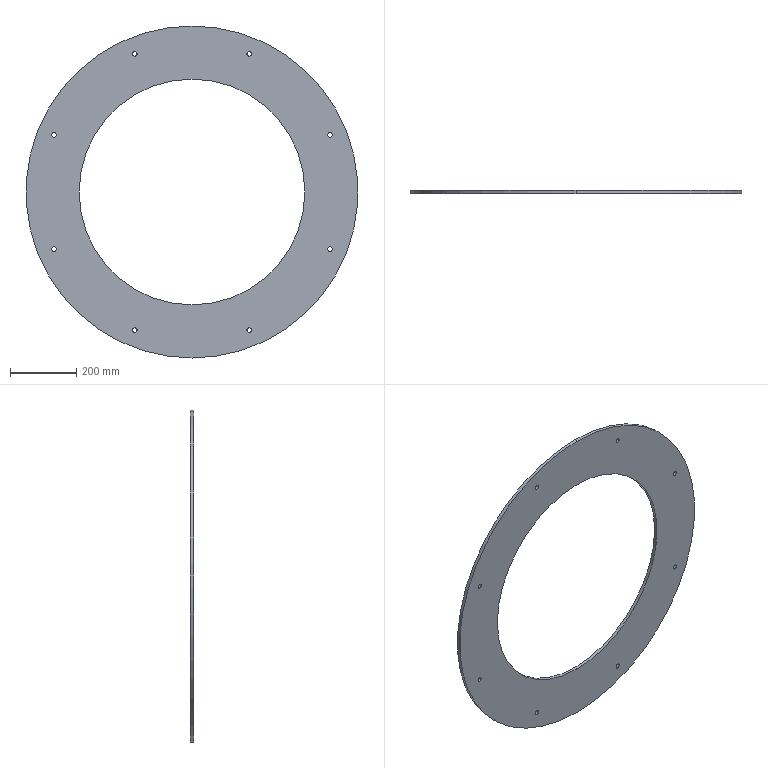Part | SolidWorks | features Extrusion 1, HoleWzd 1 | 1 solid | 22 faces | box 1000 x 10 x 1000 mm | volume 4210849 mm3 | cylinder 20 | plane 2 | commonest cylinder face diameters 13.5 x16 680 x2 1000 x2
STEP:
#1=CARTESIAN_POINT('',(172.208,-5.,-422.496));
#2=VERTEX_POINT('',#1);
#3=CARTESIAN_POINT('',(172.208,-5.,-408.996));
#4=VERTEX_POINT('',#3);
#5=CARTESIAN_POINT('',(172.208,-5.,-415.746));
#6=DIRECTION('',(0.,1.,0.));
#7=DIRECTION('',(0.,0.,1.));
#8=AXIS2_PLACEMENT_3D('',#5,#6,#7);
#9=CIRCLE('',#8,6.75);
#10=EDGE_CURVE('',#2,#4,#9,.T.);
#11=ORIENTED_EDGE('',*,*,#10,.F.);
#12=CARTESIAN_POINT('',(172.208,5.,-422.496));
#13=VERTEX_POINT('',#12);
#14=CARTESIAN_POINT('',(172.208,5.,-422.496));
#15=DIRECTION('',(0.,1.,0.));
#16=VECTOR('',#15,1000.);
#17=LINE('',#14,#16);
#18=EDGE_CURVE('',#2,#13,#17,.T.);
#19=ORIENTED_EDGE('',*,*,#18,.T.);
#20=CARTESIAN_POINT('',(172.208,5.,-408.996));
#21=VERTEX_POINT('',#20);
#22=CARTESIAN_POINT('',(172.208,5.,-415.746));
#23=DIRECTION('',(0.,1.,0.));
#24=DIRECTION('',(0.,0.,1.));
#25=AXIS2_PLACEMENT_3D('',#22,#23,#24);
#26=CIRCLE('',#25,6.75);
#27=EDGE_CURVE('',#13,#21,#26,.T.);
#28=ORIENTED_EDGE('',*,*,#27,.T.);
#29=CARTESIAN_POINT('',(172.208,5.,-408.996));
#30=DIRECTION('',(0.,1.,0.));
#31=VECTOR('',#30,1000.);
#32=LINE('',#29,#31);
#33=EDGE_CURVE('',#4,#21,#32,.T.);
#34=ORIENTED_EDGE('',*,*,#33,.F.);
#35=EDGE_LOOP('',(#11,#19,#28,#34));
#36=FACE_OUTER_BOUND('',#35,.T.);
#37=CARTESIAN_POINT('',(172.208,5.,-415.746));
#38=DIRECTION('',(0.,1.,0.));
#39=DIRECTION('',(0.,0.,1.));
#40=AXIS2_PLACEMENT_3D('',#37,#38,#39);
#41=CYLINDRICAL_SURFACE('',#40,6.75);
#42=ADVANCED_FACE('',(#36),#41,.F.);
#43=CARTESIAN_POINT('',(415.746,-5.,-178.958));
#44=VERTEX_POINT('',#43);
#45=CARTESIAN_POINT('',(415.746,-5.,-165.458));
#46=VERTEX_POINT('',#45);
#47=CARTESIAN_POINT('',(415.746,-5.,-172.208));
#48=DIRECTION('',(0.,1.,0.));
#49=DIRECTION('',(0.,0.,1.));
#50=AXIS2_PLACEMENT_3D('',#47,#48,#49);
#51=CIRCLE('',#50,6.75);
#52=EDGE_CURVE('',#44,#46,#51,.T.);
#53=ORIENTED_EDGE('',*,*,#52,.F.);
#54=CARTESIAN_POINT('',(415.746,5.,-178.958));
#55=VERTEX_POINT('',#54);
#56=CARTESIAN_POINT('',(415.746,5.,-178.958));
#57=DIRECTION('',(0.,1.,0.));
#58=VECTOR('',#57,1000.);
#59=LINE('',#56,#58);
#60=EDGE_CURVE('',#44,#55,#59,.T.);
#61=ORIENTED_EDGE('',*,*,#60,.T.);
#62=CARTESIAN_POINT('',(415.746,5.,-165.458));
#63=VERTEX_POINT('',#62);
#64=CARTESIAN_POINT('',(415.746,5.,-172.208));
#65=DIRECTION('',(0.,1.,0.));
#66=DIRECTION('',(0.,0.,1.));
#67=AXIS2_PLACEMENT_3D('',#64,#65,#66);
#68=CIRCLE('',#67,6.75);
#69=EDGE_CURVE('',#55,#63,#68,.T.);
#70=ORIENTED_EDGE('',*,*,#69,.T.);
#71=CARTESIAN_POINT('',(415.746,5.,-165.458));
#72=DIRECTION('',(0.,1.,0.));
#73=VECTOR('',#72,1000.);
#74=LINE('',#71,#73);
#75=EDGE_CURVE('',#46,#63,#74,.T.);
#76=ORIENTED_EDGE('',*,*,#75,.F.);
#77=EDGE_LOOP('',(#53,#61,#70,#76));
#78=FACE_OUTER_BOUND('',#77,.T.);
#79=CARTESIAN_POINT('',(415.746,5.,-172.208));
#80=DIRECTION('',(0.,1.,0.));
#81=DIRECTION('',(0.,0.,1.));
#82=AXIS2_PLACEMENT_3D('',#79,#80,#81);
#83=CYLINDRICAL_SURFACE('',#82,6.75);
#84=ADVANCED_FACE('',(#78),#83,.F.);
#85=CARTESIAN_POINT('',(415.746,-5.,165.458));
#86=VERTEX_POINT('',#85);
#87=CARTESIAN_POINT('',(415.746,-5.,178.958));
#88=VERTEX_POINT('',#87);
#89=CARTESIAN_POINT('',(415.746,-5.,172.208));
#90=DIRECTION('',(0.,1.,0.));
#91=DIRECTION('',(0.,0.,1.));
#92=AXIS2_PLACEMENT_3D('',#89,#90,#91);
#93=CIRCLE('',#92,6.75);
#94=EDGE_CURVE('',#86,#88,#93,.T.);
#95=ORIENTED_EDGE('',*,*,#94,.F.);
#96=CARTESIAN_POINT('',(415.746,5.,165.458));
#97=VERTEX_POINT('',#96);
#98=CARTESIAN_POINT('',(415.746,5.,165.458));
#99=DIRECTION('',(0.,1.,0.));
#100=VECTOR('',#99,1000.);
#101=LINE('',#98,#100);
#102=EDGE_CURVE('',#86,#97,#101,.T.);
#103=ORIENTED_EDGE('',*,*,#102,.T.);
#104=CARTESIAN_POINT('',(415.746,5.,178.958));
#105=VERTEX_POINT('',#104);
#106=CARTESIAN_POINT('',(415.746,5.,172.208));
#107=DIRECTION('',(0.,1.,0.));
#108=DIRECTION('',(0.,0.,1.));
#109=AXIS2_PLACEMENT_3D('',#106,#107,#108);
#110=CIRCLE('',#109,6.75);
#111=EDGE_CURVE('',#97,#105,#110,.T.);
#112=ORIENTED_EDGE('',*,*,#111,.T.);
#113=CARTESIAN_POINT('',(415.746,5.,178.958));
#114=DIRECTION('',(0.,1.,0.));
#115=VECTOR('',#114,1000.);
#116=LINE('',#113,#115);
#117=EDGE_CURVE('',#88,#105,#116,.T.);
#118=ORIENTED_EDGE('',*,*,#117,.F.);
#119=EDGE_LOOP('',(#95,#103,#112,#118));
#120=FACE_OUTER_BOUND('',#119,.T.);
#121=CARTESIAN_POINT('',(415.746,5.,172.208));
#122=DIRECTION('',(0.,1.,0.));
#123=DIRECTION('',(0.,0.,1.));
#124=AXIS2_PLACEMENT_3D('',#121,#122,#123);
#125=CYLINDRICAL_SURFACE('',#124,6.75);
#126=ADVANCED_FACE('',(#120),#125,.F.);
#127=CARTESIAN_POINT('',(172.208,-5.,408.996));
#128=VERTEX_POINT('',#127);
#129=CARTESIAN_POINT('',(172.208,-5.,422.496));
#130=VERTEX_POINT('',#129);
#131=CARTESIAN_POINT('',(172.208,-5.,415.746));
#132=DIRECTION('',(0.,1.,0.));
#133=DIRECTION('',(0.,0.,1.));
#134=AXIS2_PLACEMENT_3D('',#131,#132,#133);
#135=CIRCLE('',#134,6.75);
#136=EDGE_CURVE('',#128,#130,#135,.T.);
#137=ORIENTED_EDGE('',*,*,#136,.F.);
#138=CARTESIAN_POINT('',(172.208,5.,408.996));
#139=VERTEX_POINT('',#138);
#140=CARTESIAN_POINT('',(172.208,5.,408.996));
#141=DIRECTION('',(0.,1.,0.));
#142=VECTOR('',#141,1000.);
#143=LINE('',#140,#142);
#144=EDGE_CURVE('',#128,#139,#143,.T.);
#145=ORIENTED_EDGE('',*,*,#144,.T.);
#146=CARTESIAN_POINT('',(172.208,5.,422.496));
#147=VERTEX_POINT('',#146);
#148=CARTESIAN_POINT('',(172.208,5.,415.746));
#149=DIRECTION('',(0.,1.,0.));
#150=DIRECTION('',(0.,0.,1.));
#151=AXIS2_PLACEMENT_3D('',#148,#149,#150);
#152=CIRCLE('',#151,6.75);
#153=EDGE_CURVE('',#139,#147,#152,.T.);
#154=ORIENTED_EDGE('',*,*,#153,.T.);
#155=CARTESIAN_POINT('',(172.208,5.,422.496));
#156=DIRECTION('',(0.,1.,0.));
#157=VECTOR('',#156,1000.);
#158=LINE('',#155,#157);
#159=EDGE_CURVE('',#130,#147,#158,.T.);
#160=ORIENTED_EDGE('',*,*,#159,.F.);
#161=EDGE_LOOP('',(#137,#145,#154,#160));
#162=FACE_OUTER_BOUND('',#161,.T.);
#163=CARTESIAN_POINT('',(172.208,5.,415.746));
#164=DIRECTION('',(0.,1.,0.));
#165=DIRECTION('',(0.,0.,1.));
#166=AXIS2_PLACEMENT_3D('',#163,#164,#165);
#167=CYLINDRICAL_SURFACE('',#166,6.75);
#168=ADVANCED_FACE('',(#162),#167,.F.);
#169=CARTESIAN_POINT('',(-172.208,-5.,408.996));
#170=VERTEX_POINT('',#169);
#171=CARTESIAN_POINT('',(-172.208,-5.,422.496));
#172=VERTEX_POINT('',#171);
#173=CARTESIAN_POINT('',(-172.208,-5.,415.746));
#174=DIRECTION('',(0.,1.,0.));
#175=DIRECTION('',(0.,0.,1.));
#176=AXIS2_PLACEMENT_3D('',#173,#174,#175);
#177=CIRCLE('',#176,6.75);
#178=EDGE_CURVE('',#170,#172,#177,.T.);
#179=ORIENTED_EDGE('',*,*,#178,.F.);
#180=CARTESIAN_POINT('',(-172.208,5.,408.996));
#181=VERTEX_POINT('',#180);
#182=CARTESIAN_POINT('',(-172.208,5.,408.996));
#183=DIRECTION('',(0.,1.,0.));
#184=VECTOR('',#183,1000.);
#185=LINE('',#182,#184);
#186=EDGE_CURVE('',#170,#181,#185,.T.);
#187=ORIENTED_EDGE('',*,*,#186,.T.);
#188=CARTESIAN_POINT('',(-172.208,5.,422.496));
#189=VERTEX_POINT('',#188);
#190=CARTESIAN_POINT('',(-172.208,5.,415.746));
#191=DIRECTION('',(0.,1.,0.));
#192=DIRECTION('',(0.,0.,1.));
#193=AXIS2_PLACEMENT_3D('',#190,#191,#192);
#194=CIRCLE('',#193,6.75);
#195=EDGE_CURVE('',#181,#189,#194,.T.);
#196=ORIENTED_EDGE('',*,*,#195,.T.);
#197=CARTESIAN_POINT('',(-172.208,5.,422.496));
#198=DIRECTION('',(0.,1.,0.));
#199=VECTOR('',#198,1000.);
#200=LINE('',#197,#199);
#201=EDGE_CURVE('',#172,#189,#200,.T.);
#202=ORIENTED_EDGE('',*,*,#201,.F.);
#203=EDGE_LOOP('',(#179,#187,#196,#202));
#204=FACE_OUTER_BOUND('',#203,.T.);
#205=CARTESIAN_POINT('',(-172.208,5.,415.746));
#206=DIRECTION('',(0.,1.,0.));
#207=DIRECTION('',(0.,0.,1.));
#208=AXIS2_PLACEMENT_3D('',#205,#206,#207);
#209=CYLINDRICAL_SURFACE('',#208,6.75);
#210=ADVANCED_FACE('',(#204),#209,.F.);
#211=CARTESIAN_POINT('',(-415.746,-5.,165.458));
#212=VERTEX_POINT('',#211);
#213=CARTESIAN_POINT('',(-415.746,-5.,178.958));
#214=VERTEX_POINT('',#213);
#215=CARTESIAN_POINT('',(-415.746,-5.,172.208));
#216=DIRECTION('',(0.,1.,0.));
#217=DIRECTION('',(0.,0.,1.));
#218=AXIS2_PLACEMENT_3D('',#215,#216,#217);
#219=CIRCLE('',#218,6.75);
#220=EDGE_CURVE('',#212,#214,#219,.T.);
#221=ORIENTED_EDGE('',*,*,#220,.F.);
#222=CARTESIAN_POINT('',(-415.746,5.,165.458));
#223=VERTEX_POINT('',#222);
#224=CARTESIAN_POINT('',(-415.746,5.,165.458));
#225=DIRECTION('',(0.,1.,0.));
#226=VECTOR('',#225,1000.);
#227=LINE('',#224,#226);
#228=EDGE_CURVE('',#212,#223,#227,.T.);
#229=ORIENTED_EDGE('',*,*,#228,.T.);
#230=CARTESIAN_POINT('',(-415.746,5.,178.958));
#231=VERTEX_POINT('',#230);
#232=CARTESIAN_POINT('',(-415.746,5.,172.208));
#233=DIRECTION('',(0.,1.,0.));
#234=DIRECTION('',(0.,0.,1.));
#235=AXIS2_PLACEMENT_3D('',#232,#233,#234);
#236=CIRCLE('',#235,6.75);
#237=EDGE_CURVE('',#223,#231,#236,.T.);
#238=ORIENTED_EDGE('',*,*,#237,.T.);
#239=CARTESIAN_POINT('',(-415.746,5.,178.958));
#240=DIRECTION('',(0.,1.,0.));
#241=VECTOR('',#240,1000.);
#242=LINE('',#239,#241);
#243=EDGE_CURVE('',#214,#231,#242,.T.);
#244=ORIENTED_EDGE('',*,*,#243,.F.);
#245=EDGE_LOOP('',(#221,#229,#238,#244));
#246=FACE_OUTER_BOUND('',#245,.T.);
#247=CARTESIAN_POINT('',(-415.746,5.,172.208));
#248=DIRECTION('',(0.,1.,0.));
#249=DIRECTION('',(0.,0.,1.));
#250=AXIS2_PLACEMENT_3D('',#247,#248,#249);
#251=CYLINDRICAL_SURFACE('',#250,6.75);
#252=ADVANCED_FACE('',(#246),#251,.F.);
#253=CARTESIAN_POINT('',(-415.746,-5.,-178.958));
#254=VERTEX_POINT('',#253);
#255=CARTESIAN_POINT('',(-415.746,-5.,-165.458));
#256=VERTEX_POINT('',#255);
#257=CARTESIAN_POINT('',(-415.746,-5.,-172.208));
#258=DIRECTION('',(0.,1.,0.));
#259=DIRECTION('',(0.,0.,1.));
#260=AXIS2_PLACEMENT_3D('',#257,#258,#259);
#261=CIRCLE('',#260,6.75);
#262=EDGE_CURVE('',#254,#256,#261,.T.);
#263=ORIENTED_EDGE('',*,*,#262,.F.);
#264=CARTESIAN_POINT('',(-415.746,5.,-178.958));
#265=VERTEX_POINT('',#264);
#266=CARTESIAN_POINT('',(-415.746,5.,-178.958));
#267=DIRECTION('',(0.,1.,0.));
#268=VECTOR('',#267,1000.);
#269=LINE('',#266,#268);
#270=EDGE_CURVE('',#254,#265,#269,.T.);
#271=ORIENTED_EDGE('',*,*,#270,.T.);
#272=CARTESIAN_POINT('',(-415.746,5.,-165.458));
#273=VERTEX_POINT('',#272);
#274=CARTESIAN_POINT('',(-415.746,5.,-172.208));
#275=DIRECTION('',(0.,1.,0.));
#276=DIRECTION('',(0.,0.,1.));
#277=AXIS2_PLACEMENT_3D('',#274,#275,#276);
#278=CIRCLE('',#277,6.75);
#279=EDGE_CURVE('',#265,#273,#278,.T.);
#280=ORIENTED_EDGE('',*,*,#279,.T.);
#281=CARTESIAN_POINT('',(-415.746,5.,-165.458));
#282=DIRECTION('',(0.,1.,0.));
#283=VECTOR('',#282,1000.);
#284=LINE('',#281,#283);
#285=EDGE_CURVE('',#256,#273,#284,.T.);
#286=ORIENTED_EDGE('',*,*,#285,.F.);
#287=EDGE_LOOP('',(#263,#271,#280,#286));
#288=FACE_OUTER_BOUND('',#287,.T.);
#289=CARTESIAN_POINT('',(-415.746,5.,-172.208));
#290=DIRECTION('',(0.,1.,0.));
#291=DIRECTION('',(0.,0.,1.));
#292=AXIS2_PLACEMENT_3D('',#289,#290,#291);
#293=CYLINDRICAL_SURFACE('',#292,6.75);
#294=ADVANCED_FACE('',(#288),#293,.F.);
#295=CARTESIAN_POINT('',(-172.208,-5.,-422.496));
#296=VERTEX_POINT('',#295);
#297=CARTESIAN_POINT('',(-172.208,-5.,-408.996));
#298=VERTEX_POINT('',#297);
#299=CARTESIAN_POINT('',(-172.208,-5.,-415.746));
#300=DIRECTION('',(0.,1.,0.));
#301=DIRECTION('',(0.,0.,1.));
#302=AXIS2_PLACEMENT_3D('',#299,#300,#301);
#303=CIRCLE('',#302,6.75);
#304=EDGE_CURVE('',#296,#298,#303,.T.);
#305=ORIENTED_EDGE('',*,*,#304,.F.);
#306=CARTESIAN_POINT('',(-172.208,5.,-422.496));
#307=VERTEX_POINT('',#306);
#308=CARTESIAN_POINT('',(-172.208,5.,-422.496));
#309=DIRECTION('',(0.,1.,0.));
#310=VECTOR('',#309,1000.);
#311=LINE('',#308,#310);
#312=EDGE_CURVE('',#296,#307,#311,.T.);
#313=ORIENTED_EDGE('',*,*,#312,.T.);
#314=CARTESIAN_POINT('',(-172.208,5.,-408.996));
#315=VERTEX_POINT('',#314);
#316=CARTESIAN_POINT('',(-172.208,5.,-415.746));
#317=DIRECTION('',(0.,1.,0.));
#318=DIRECTION('',(0.,0.,1.));
#319=AXIS2_PLACEMENT_3D('',#316,#317,#318);
#320=CIRCLE('',#319,6.75);
#321=EDGE_CURVE('',#307,#315,#320,.T.);
#322=ORIENTED_EDGE('',*,*,#321,.T.);
#323=CARTESIAN_POINT('',(-172.208,5.,-408.996));
#324=DIRECTION('',(0.,1.,0.));
#325=VECTOR('',#324,1000.);
#326=LINE('',#323,#325);
#327=EDGE_CURVE('',#298,#315,#326,.T.);
#328=ORIENTED_EDGE('',*,*,#327,.F.);
#329=EDGE_LOOP('',(#305,#313,#322,#328));
#330=FACE_OUTER_BOUND('',#329,.T.);
#331=CARTESIAN_POINT('',(-172.208,5.,-415.746));
#332=DIRECTION('',(0.,1.,0.));
#333=DIRECTION('',(0.,0.,1.));
#334=AXIS2_PLACEMENT_3D('',#331,#332,#333);
#335=CYLINDRICAL_SURFACE('',#334,6.75);
#336=ADVANCED_FACE('',(#330),#335,.F.);
#337=CARTESIAN_POINT('',(0.,5.,-340.));
#338=VERTEX_POINT('',#337);
#339=CARTESIAN_POINT('',(0.,5.,340.));
#340=VERTEX_POINT('',#339);
#341=CARTESIAN_POINT('',(0.,5.,0.));
#342=DIRECTION('',(0.,1.,0.));
#343=DIRECTION('',(0.,0.,1.));
#344=AXIS2_PLACEMENT_3D('',#341,#342,#343);
#345=CIRCLE('',#344,340.);
#346=EDGE_CURVE('',#338,#340,#345,.T.);
#347=ORIENTED_EDGE('',*,*,#346,.T.);
#348=CARTESIAN_POINT('',(0.,-5.,340.));
#349=VERTEX_POINT('',#348);
#350=CARTESIAN_POINT('',(0.,5.,340.));
#351=DIRECTION('',(0.,-1.,0.));
#352=VECTOR('',#351,1000.);
#353=LINE('',#350,#352);
#354=EDGE_CURVE('',#340,#349,#353,.T.);
#355=ORIENTED_EDGE('',*,*,#354,.T.);
#356=CARTESIAN_POINT('',(0.,-5.,-340.));
#357=VERTEX_POINT('',#356);
#358=CARTESIAN_POINT('',(0.,-5.,0.));
#359=DIRECTION('',(0.,1.,0.));
#360=DIRECTION('',(0.,0.,1.));
#361=AXIS2_PLACEMENT_3D('',#358,#359,#360);
#362=CIRCLE('',#361,340.);
#363=EDGE_CURVE('',#357,#349,#362,.T.);
#364=ORIENTED_EDGE('',*,*,#363,.F.);
#365=CARTESIAN_POINT('',(0.,5.,-340.));
#366=DIRECTION('',(0.,-1.,0.));
#367=VECTOR('',#366,1000.);
#368=LINE('',#365,#367);
#369=EDGE_CURVE('',#338,#357,#368,.T.);
#370=ORIENTED_EDGE('',*,*,#369,.F.);
#371=EDGE_LOOP('',(#347,#355,#364,#370));
#372=FACE_OUTER_BOUND('',#371,.T.);
#373=CARTESIAN_POINT('',(0.,5.,0.));
#374=DIRECTION('',(0.,-1.,0.));
#375=DIRECTION('',(0.,0.,-1.));
#376=AXIS2_PLACEMENT_3D('',#373,#374,#375);
#377=CYLINDRICAL_SURFACE('',#376,340.);
#378=ADVANCED_FACE('',(#372),#377,.F.);
#379=CARTESIAN_POINT('',(0.,5.,500.));
#380=VERTEX_POINT('',#379);
#381=CARTESIAN_POINT('',(0.,5.,-500.));
#382=VERTEX_POINT('',#381);
#383=CARTESIAN_POINT('',(0.,5.,0.));
#384=DIRECTION('',(0.,1.,0.));
#385=DIRECTION('',(0.,0.,1.));
#386=AXIS2_PLACEMENT_3D('',#383,#384,#385);
#387=CIRCLE('',#386,500.);
#388=EDGE_CURVE('',#380,#382,#387,.T.);
#389=ORIENTED_EDGE('',*,*,#388,.F.);
#390=CARTESIAN_POINT('',(0.,-5.,500.));
#391=VERTEX_POINT('',#390);
#392=CARTESIAN_POINT('',(0.,5.,500.));
#393=DIRECTION('',(0.,-1.,0.));
#394=VECTOR('',#393,1000.);
#395=LINE('',#392,#394);
#396=EDGE_CURVE('',#380,#391,#395,.T.);
#397=ORIENTED_EDGE('',*,*,#396,.T.);
#398=CARTESIAN_POINT('',(0.,-5.,-500.));
#399=VERTEX_POINT('',#398);
#400=CARTESIAN_POINT('',(0.,-5.,0.));
#401=DIRECTION('',(0.,1.,0.));
#402=DIRECTION('',(0.,0.,1.));
#403=AXIS2_PLACEMENT_3D('',#400,#401,#402);
#404=CIRCLE('',#403,500.);
#405=EDGE_CURVE('',#391,#399,#404,.T.);
#406=ORIENTED_EDGE('',*,*,#405,.T.);
#407=CARTESIAN_POINT('',(0.,5.,-500.));
#408=DIRECTION('',(0.,-1.,0.));
#409=VECTOR('',#408,1000.);
#410=LINE('',#407,#409);
#411=EDGE_CURVE('',#382,#399,#410,.T.);
#412=ORIENTED_EDGE('',*,*,#411,.F.);
#413=EDGE_LOOP('',(#389,#397,#406,#412));
#414=FACE_OUTER_BOUND('',#413,.T.);
#415=CARTESIAN_POINT('',(0.,5.,0.));
#416=DIRECTION('',(0.,-1.,0.));
#417=DIRECTION('',(0.,0.,-1.));
#418=AXIS2_PLACEMENT_3D('',#415,#416,#417);
#419=CYLINDRICAL_SURFACE('',#418,500.);
#420=ADVANCED_FACE('',(#414),#419,.T.);
#421=CARTESIAN_POINT('',(172.208,5.,-415.746));
#422=DIRECTION('',(0.,1.,0.));
#423=DIRECTION('',(0.,0.,1.));
#424=AXIS2_PLACEMENT_3D('',#421,#422,#423);
#425=CIRCLE('',#424,6.75);
#426=EDGE_CURVE('',#21,#13,#425,.T.);
#427=ORIENTED_EDGE('',*,*,#426,.F.);
#428=ORIENTED_EDGE('',*,*,#27,.F.);
#429=EDGE_LOOP('',(#427,#428));
#430=FACE_BOUND('',#429,.T.);
#431=CARTESIAN_POINT('',(415.746,5.,-172.208));
#432=DIRECTION('',(0.,1.,0.));
#433=DIRECTION('',(0.,0.,1.));
#434=AXIS2_PLACEMENT_3D('',#431,#432,#433);
#435=CIRCLE('',#434,6.75);
#436=EDGE_CURVE('',#63,#55,#435,.T.);
#437=ORIENTED_EDGE('',*,*,#436,.F.);
#438=ORIENTED_EDGE('',*,*,#69,.F.);
#439=EDGE_LOOP('',(#437,#438));
#440=FACE_BOUND('',#439,.T.);
#441=CARTESIAN_POINT('',(415.746,5.,172.208));
#442=DIRECTION('',(0.,1.,0.));
#443=DIRECTION('',(0.,0.,1.));
#444=AXIS2_PLACEMENT_3D('',#441,#442,#443);
#445=CIRCLE('',#444,6.75);
#446=EDGE_CURVE('',#105,#97,#445,.T.);
#447=ORIENTED_EDGE('',*,*,#446,.F.);
#448=ORIENTED_EDGE('',*,*,#111,.F.);
#449=EDGE_LOOP('',(#447,#448));
#450=FACE_BOUND('',#449,.T.);
#451=CARTESIAN_POINT('',(172.208,5.,415.746));
#452=DIRECTION('',(0.,1.,0.));
#453=DIRECTION('',(0.,0.,1.));
#454=AXIS2_PLACEMENT_3D('',#451,#452,#453);
#455=CIRCLE('',#454,6.75);
#456=EDGE_CURVE('',#147,#139,#455,.T.);
#457=ORIENTED_EDGE('',*,*,#456,.F.);
#458=ORIENTED_EDGE('',*,*,#153,.F.);
#459=EDGE_LOOP('',(#457,#458));
#460=FACE_BOUND('',#459,.T.);
#461=CARTESIAN_POINT('',(-172.208,5.,415.746));
#462=DIRECTION('',(0.,1.,0.));
#463=DIRECTION('',(0.,0.,1.));
#464=AXIS2_PLACEMENT_3D('',#461,#462,#463);
#465=CIRCLE('',#464,6.75);
#466=EDGE_CURVE('',#189,#181,#465,.T.);
#467=ORIENTED_EDGE('',*,*,#466,.F.);
#468=ORIENTED_EDGE('',*,*,#195,.F.);
#469=EDGE_LOOP('',(#467,#468));
#470=FACE_BOUND('',#469,.T.);
#471=CARTESIAN_POINT('',(-415.746,5.,172.208));
#472=DIRECTION('',(0.,1.,0.));
#473=DIRECTION('',(0.,0.,1.));
#474=AXIS2_PLACEMENT_3D('',#471,#472,#473);
#475=CIRCLE('',#474,6.75);
#476=EDGE_CURVE('',#231,#223,#475,.T.);
#477=ORIENTED_EDGE('',*,*,#476,.F.);
#478=ORIENTED_EDGE('',*,*,#237,.F.);
#479=EDGE_LOOP('',(#477,#478));
#480=FACE_BOUND('',#479,.T.);
#481=CARTESIAN_POINT('',(-415.746,5.,-172.208));
#482=DIRECTION('',(0.,1.,0.));
#483=DIRECTION('',(0.,0.,1.));
#484=AXIS2_PLACEMENT_3D('',#481,#482,#483);
#485=CIRCLE('',#484,6.75);
#486=EDGE_CURVE('',#273,#265,#485,.T.);
#487=ORIENTED_EDGE('',*,*,#486,.F.);
#488=ORIENTED_EDGE('',*,*,#279,.F.);
#489=EDGE_LOOP('',(#487,#488));
#490=FACE_BOUND('',#489,.T.);
#491=CARTESIAN_POINT('',(-172.208,5.,-415.746));
#492=DIRECTION('',(0.,1.,0.));
#493=DIRECTION('',(0.,0.,1.));
#494=AXIS2_PLACEMENT_3D('',#491,#492,#493);
#495=CIRCLE('',#494,6.75);
#496=EDGE_CURVE('',#315,#307,#495,.T.);
#497=ORIENTED_EDGE('',*,*,#496,.F.);
#498=ORIENTED_EDGE('',*,*,#321,.F.);
#499=EDGE_LOOP('',(#497,#498));
#500=FACE_BOUND('',#499,.T.);
#501=CARTESIAN_POINT('',(0.,5.,0.));
#502=DIRECTION('',(0.,1.,0.));
#503=DIRECTION('',(0.,0.,1.));
#504=AXIS2_PLACEMENT_3D('',#501,#502,#503);
#505=CIRCLE('',#504,500.);
#506=EDGE_CURVE('',#382,#380,#505,.T.);
#507=ORIENTED_EDGE('',*,*,#506,.T.);
#508=ORIENTED_EDGE('',*,*,#388,.T.);
#509=EDGE_LOOP('',(#507,#508));
#510=FACE_OUTER_BOUND('',#509,.T.);
#511=ORIENTED_EDGE('',*,*,#346,.F.);
#512=CARTESIAN_POINT('',(0.,5.,0.));
#513=DIRECTION('',(0.,1.,0.));
#514=DIRECTION('',(0.,0.,1.));
#515=AXIS2_PLACEMENT_3D('',#512,#513,#514);
#516=CIRCLE('',#515,340.);
#517=EDGE_CURVE('',#340,#338,#516,.T.);
#518=ORIENTED_EDGE('',*,*,#517,.F.);
#519=EDGE_LOOP('',(#511,#518));
#520=FACE_BOUND('',#519,.T.);
#521=CARTESIAN_POINT('',(0.,5.,0.));
#522=DIRECTION('',(0.,1.,0.));
#523=DIRECTION('',(0.,0.,1.));
#524=AXIS2_PLACEMENT_3D('',#521,#522,#523);
#525=PLANE('',#524);
#526=ADVANCED_FACE('',(#430,#440,#450,#460,#470,#480,#490,#500,#510,#520),#525,.T.);
#527=CARTESIAN_POINT('',(172.208,-5.,-415.746));
#528=DIRECTION('',(0.,1.,0.));
#529=DIRECTION('',(0.,0.,1.));
#530=AXIS2_PLACEMENT_3D('',#527,#528,#529);
#531=CIRCLE('',#530,6.75);
#532=EDGE_CURVE('',#4,#2,#531,.T.);
#533=ORIENTED_EDGE('',*,*,#532,.T.);
#534=ORIENTED_EDGE('',*,*,#10,.T.);
#535=EDGE_LOOP('',(#533,#534));
#536=FACE_BOUND('',#535,.T.);
#537=CARTESIAN_POINT('',(415.746,-5.,-172.208));
#538=DIRECTION('',(0.,1.,0.));
#539=DIRECTION('',(0.,0.,1.));
#540=AXIS2_PLACEMENT_3D('',#537,#538,#539);
#541=CIRCLE('',#540,6.75);
#542=EDGE_CURVE('',#46,#44,#541,.T.);
#543=ORIENTED_EDGE('',*,*,#542,.T.);
#544=ORIENTED_EDGE('',*,*,#52,.T.);
#545=EDGE_LOOP('',(#543,#544));
#546=FACE_BOUND('',#545,.T.);
#547=CARTESIAN_POINT('',(415.746,-5.,172.208));
#548=DIRECTION('',(0.,1.,0.));
#549=DIRECTION('',(0.,0.,1.));
#550=AXIS2_PLACEMENT_3D('',#547,#548,#549);
#551=CIRCLE('',#550,6.75);
#552=EDGE_CURVE('',#88,#86,#551,.T.);
#553=ORIENTED_EDGE('',*,*,#552,.T.);
#554=ORIENTED_EDGE('',*,*,#94,.T.);
#555=EDGE_LOOP('',(#553,#554));
#556=FACE_BOUND('',#555,.T.);
#557=CARTESIAN_POINT('',(172.208,-5.,415.746));
#558=DIRECTION('',(0.,1.,0.));
#559=DIRECTION('',(0.,0.,1.));
#560=AXIS2_PLACEMENT_3D('',#557,#558,#559);
#561=CIRCLE('',#560,6.75);
#562=EDGE_CURVE('',#130,#128,#561,.T.);
#563=ORIENTED_EDGE('',*,*,#562,.T.);
#564=ORIENTED_EDGE('',*,*,#136,.T.);
#565=EDGE_LOOP('',(#563,#564));
#566=FACE_BOUND('',#565,.T.);
#567=CARTESIAN_POINT('',(-172.208,-5.,415.746));
#568=DIRECTION('',(0.,1.,0.));
#569=DIRECTION('',(0.,0.,1.));
#570=AXIS2_PLACEMENT_3D('',#567,#568,#569);
#571=CIRCLE('',#570,6.75);
#572=EDGE_CURVE('',#172,#170,#571,.T.);
#573=ORIENTED_EDGE('',*,*,#572,.T.);
#574=ORIENTED_EDGE('',*,*,#178,.T.);
#575=EDGE_LOOP('',(#573,#574));
#576=FACE_BOUND('',#575,.T.);
#577=CARTESIAN_POINT('',(-415.746,-5.,172.208));
#578=DIRECTION('',(0.,1.,0.));
#579=DIRECTION('',(0.,0.,1.));
#580=AXIS2_PLACEMENT_3D('',#577,#578,#579);
#581=CIRCLE('',#580,6.75);
#582=EDGE_CURVE('',#214,#212,#581,.T.);
#583=ORIENTED_EDGE('',*,*,#582,.T.);
#584=ORIENTED_EDGE('',*,*,#220,.T.);
#585=EDGE_LOOP('',(#583,#584));
#586=FACE_BOUND('',#585,.T.);
#587=CARTESIAN_POINT('',(-415.746,-5.,-172.208));
#588=DIRECTION('',(0.,1.,0.));
#589=DIRECTION('',(0.,0.,1.));
#590=AXIS2_PLACEMENT_3D('',#587,#588,#589);
#591=CIRCLE('',#590,6.75);
#592=EDGE_CURVE('',#256,#254,#591,.T.);
#593=ORIENTED_EDGE('',*,*,#592,.T.);
#594=ORIENTED_EDGE('',*,*,#262,.T.);
#595=EDGE_LOOP('',(#593,#594));
#596=FACE_BOUND('',#595,.T.);
#597=CARTESIAN_POINT('',(-172.208,-5.,-415.746));
#598=DIRECTION('',(0.,1.,0.));
#599=DIRECTION('',(0.,0.,1.));
#600=AXIS2_PLACEMENT_3D('',#597,#598,#599);
#601=CIRCLE('',#600,6.75);
#602=EDGE_CURVE('',#298,#296,#601,.T.);
#603=ORIENTED_EDGE('',*,*,#602,.T.);
#604=ORIENTED_EDGE('',*,*,#304,.T.);
#605=EDGE_LOOP('',(#603,#604));
#606=FACE_BOUND('',#605,.T.);
#607=CARTESIAN_POINT('',(0.,-5.,0.));
#608=DIRECTION('',(0.,1.,0.));
#609=DIRECTION('',(0.,0.,1.));
#610=AXIS2_PLACEMENT_3D('',#607,#608,#609);
#611=CIRCLE('',#610,500.);
#612=EDGE_CURVE('',#399,#391,#611,.T.);
#613=ORIENTED_EDGE('',*,*,#612,.F.);
#614=ORIENTED_EDGE('',*,*,#405,.F.);
#615=EDGE_LOOP('',(#613,#614));
#616=FACE_OUTER_BOUND('',#615,.T.);
#617=ORIENTED_EDGE('',*,*,#363,.T.);
#618=CARTESIAN_POINT('',(0.,-5.,0.));
#619=DIRECTION('',(0.,1.,0.));
#620=DIRECTION('',(0.,0.,1.));
#621=AXIS2_PLACEMENT_3D('',#618,#619,#620);
#622=CIRCLE('',#621,340.);
#623=EDGE_CURVE('',#349,#357,#622,.T.);
#624=ORIENTED_EDGE('',*,*,#623,.T.);
#625=EDGE_LOOP('',(#617,#624));
#626=FACE_BOUND('',#625,.T.);
#627=CARTESIAN_POINT('',(0.,-5.,0.));
#628=DIRECTION('',(0.,1.,0.));
#629=DIRECTION('',(0.,0.,1.));
#630=AXIS2_PLACEMENT_3D('',#627,#628,#629);
#631=PLANE('',#630);
#632=ADVANCED_FACE('',(#536,#546,#556,#566,#576,#586,#596,#606,#616,#626),#631,.F.);
#633=ORIENTED_EDGE('',*,*,#396,.F.);
#634=ORIENTED_EDGE('',*,*,#506,.F.);
#635=ORIENTED_EDGE('',*,*,#411,.T.);
#636=ORIENTED_EDGE('',*,*,#612,.T.);
#637=EDGE_LOOP('',(#633,#634,#635,#636));
#638=FACE_OUTER_BOUND('',#637,.T.);
#639=CARTESIAN_POINT('',(0.,5.,0.));
#640=DIRECTION('',(0.,-1.,0.));
#641=DIRECTION('',(0.,0.,-1.));
#642=AXIS2_PLACEMENT_3D('',#639,#640,#641);
#643=CYLINDRICAL_SURFACE('',#642,500.);
#644=ADVANCED_FACE('',(#638),#643,.T.);
#645=ORIENTED_EDGE('',*,*,#354,.F.);
#646=ORIENTED_EDGE('',*,*,#517,.T.);
#647=ORIENTED_EDGE('',*,*,#369,.T.);
#648=ORIENTED_EDGE('',*,*,#623,.F.);
#649=EDGE_LOOP('',(#645,#646,#647,#648));
#650=FACE_OUTER_BOUND('',#649,.T.);
#651=CARTESIAN_POINT('',(0.,5.,0.));
#652=DIRECTION('',(0.,-1.,0.));
#653=DIRECTION('',(0.,0.,-1.));
#654=AXIS2_PLACEMENT_3D('',#651,#652,#653);
#655=CYLINDRICAL_SURFACE('',#654,340.);
#656=ADVANCED_FACE('',(#650),#655,.F.);
#657=ORIENTED_EDGE('',*,*,#312,.F.);
#658=ORIENTED_EDGE('',*,*,#602,.F.);
#659=ORIENTED_EDGE('',*,*,#327,.T.);
#660=ORIENTED_EDGE('',*,*,#496,.T.);
#661=EDGE_LOOP('',(#657,#658,#659,#660));
#662=FACE_OUTER_BOUND('',#661,.T.);
#663=CARTESIAN_POINT('',(-172.208,5.,-415.746));
#664=DIRECTION('',(0.,1.,0.));
#665=DIRECTION('',(0.,0.,1.));
#666=AXIS2_PLACEMENT_3D('',#663,#664,#665);
#667=CYLINDRICAL_SURFACE('',#666,6.75);
#668=ADVANCED_FACE('',(#662),#667,.F.);
#669=ORIENTED_EDGE('',*,*,#270,.F.);
#670=ORIENTED_EDGE('',*,*,#592,.F.);
#671=ORIENTED_EDGE('',*,*,#285,.T.);
#672=ORIENTED_EDGE('',*,*,#486,.T.);
#673=EDGE_LOOP('',(#669,#670,#671,#672));
#674=FACE_OUTER_BOUND('',#673,.T.);
#675=CARTESIAN_POINT('',(-415.746,5.,-172.208));
#676=DIRECTION('',(0.,1.,0.));
#677=DIRECTION('',(0.,0.,1.));
#678=AXIS2_PLACEMENT_3D('',#675,#676,#677);
#679=CYLINDRICAL_SURFACE('',#678,6.75);
#680=ADVANCED_FACE('',(#674),#679,.F.);
#681=ORIENTED_EDGE('',*,*,#228,.F.);
#682=ORIENTED_EDGE('',*,*,#582,.F.);
#683=ORIENTED_EDGE('',*,*,#243,.T.);
#684=ORIENTED_EDGE('',*,*,#476,.T.);
#685=EDGE_LOOP('',(#681,#682,#683,#684));
#686=FACE_OUTER_BOUND('',#685,.T.);
#687=CARTESIAN_POINT('',(-415.746,5.,172.208));
#688=DIRECTION('',(0.,1.,0.));
#689=DIRECTION('',(0.,0.,1.));
#690=AXIS2_PLACEMENT_3D('',#687,#688,#689);
#691=CYLINDRICAL_SURFACE('',#690,6.75);
#692=ADVANCED_FACE('',(#686),#691,.F.);
#693=ORIENTED_EDGE('',*,*,#186,.F.);
#694=ORIENTED_EDGE('',*,*,#572,.F.);
#695=ORIENTED_EDGE('',*,*,#201,.T.);
#696=ORIENTED_EDGE('',*,*,#466,.T.);
#697=EDGE_LOOP('',(#693,#694,#695,#696));
#698=FACE_OUTER_BOUND('',#697,.T.);
#699=CARTESIAN_POINT('',(-172.208,5.,415.746));
#700=DIRECTION('',(0.,1.,0.));
#701=DIRECTION('',(0.,0.,1.));
#702=AXIS2_PLACEMENT_3D('',#699,#700,#701);
#703=CYLINDRICAL_SURFACE('',#702,6.75);
#704=ADVANCED_FACE('',(#698),#703,.F.);
#705=ORIENTED_EDGE('',*,*,#144,.F.);
#706=ORIENTED_EDGE('',*,*,#562,.F.);
#707=ORIENTED_EDGE('',*,*,#159,.T.);
#708=ORIENTED_EDGE('',*,*,#456,.T.);
#709=EDGE_LOOP('',(#705,#706,#707,#708));
#710=FACE_OUTER_BOUND('',#709,.T.);
#711=CARTESIAN_POINT('',(172.208,5.,415.746));
#712=DIRECTION('',(0.,1.,0.));
#713=DIRECTION('',(0.,0.,1.));
#714=AXIS2_PLACEMENT_3D('',#711,#712,#713);
#715=CYLINDRICAL_SURFACE('',#714,6.75);
#716=ADVANCED_FACE('',(#710),#715,.F.);
#717=ORIENTED_EDGE('',*,*,#102,.F.);
#718=ORIENTED_EDGE('',*,*,#552,.F.);
#719=ORIENTED_EDGE('',*,*,#117,.T.);
#720=ORIENTED_EDGE('',*,*,#446,.T.);
#721=EDGE_LOOP('',(#717,#718,#719,#720));
#722=FACE_OUTER_BOUND('',#721,.T.);
#723=CARTESIAN_POINT('',(415.746,5.,172.208));
#724=DIRECTION('',(0.,1.,0.));
#725=DIRECTION('',(0.,0.,1.));
#726=AXIS2_PLACEMENT_3D('',#723,#724,#725);
#727=CYLINDRICAL_SURFACE('',#726,6.75);
#728=ADVANCED_FACE('',(#722),#727,.F.);
#729=ORIENTED_EDGE('',*,*,#60,.F.);
#730=ORIENTED_EDGE('',*,*,#542,.F.);
#731=ORIENTED_EDGE('',*,*,#75,.T.);
#732=ORIENTED_EDGE('',*,*,#436,.T.);
#733=EDGE_LOOP('',(#729,#730,#731,#732));
#734=FACE_OUTER_BOUND('',#733,.T.);
#735=CARTESIAN_POINT('',(415.746,5.,-172.208));
#736=DIRECTION('',(0.,1.,0.));
#737=DIRECTION('',(0.,0.,1.));
#738=AXIS2_PLACEMENT_3D('',#735,#736,#737);
#739=CYLINDRICAL_SURFACE('',#738,6.75);
#740=ADVANCED_FACE('',(#734),#739,.F.);
#741=ORIENTED_EDGE('',*,*,#18,.F.);
#742=ORIENTED_EDGE('',*,*,#532,.F.);
#743=ORIENTED_EDGE('',*,*,#33,.T.);
#744=ORIENTED_EDGE('',*,*,#426,.T.);
#745=EDGE_LOOP('',(#741,#742,#743,#744));
#746=FACE_OUTER_BOUND('',#745,.T.);
#747=CARTESIAN_POINT('',(172.208,5.,-415.746));
#748=DIRECTION('',(0.,1.,0.));
#749=DIRECTION('',(0.,0.,1.));
#750=AXIS2_PLACEMENT_3D('',#747,#748,#749);
#751=CYLINDRICAL_SURFACE('',#750,6.75);
#752=ADVANCED_FACE('',(#746),#751,.F.);
#753=CLOSED_SHELL('',(#42,#84,#126,#168,#210,#252,#294,#336,#378,#420,#526,#632,#644,#656,#668,#680,#692,#704,#716,#728,#740,#752));
#754=MANIFOLD_SOLID_BREP('',#753);
#755=CARTESIAN_POINT('',(0.,0.,0.));
#756=DIRECTION('',(0.,0.,1.));
#757=DIRECTION('',(1.,0.,0.));
#758=AXIS2_PLACEMENT_3D('',#755,#756,#757);
#759=(LENGTH_UNIT()NAMED_UNIT(*)SI_UNIT(.MILLI.,.METRE.));
#760=UNCERTAINTY_MEASURE_WITH_UNIT(LENGTH_MEASURE(0.00001),#759,'','');
#761=(NAMED_UNIT(*)PLANE_ANGLE_UNIT()SI_UNIT($,.RADIAN.));
#762=(NAMED_UNIT(*)SI_UNIT($,.STERADIAN.)SOLID_ANGLE_UNIT());
#763=(GEOMETRIC_REPRESENTATION_CONTEXT(3)GLOBAL_UNCERTAINTY_ASSIGNED_CONTEXT((#760))GLOBAL_UNIT_ASSIGNED_CONTEXT((#759,#761,#762))REPRESENTATION_CONTEXT('',''));
#764=ADVANCED_BREP_SHAPE_REPRESENTATION('',(#754,#758),#763);